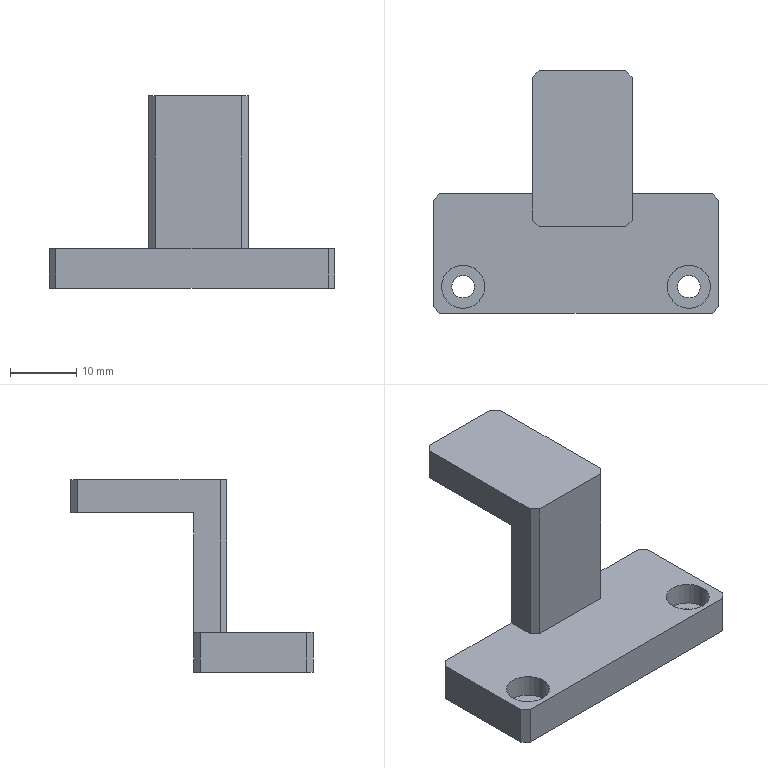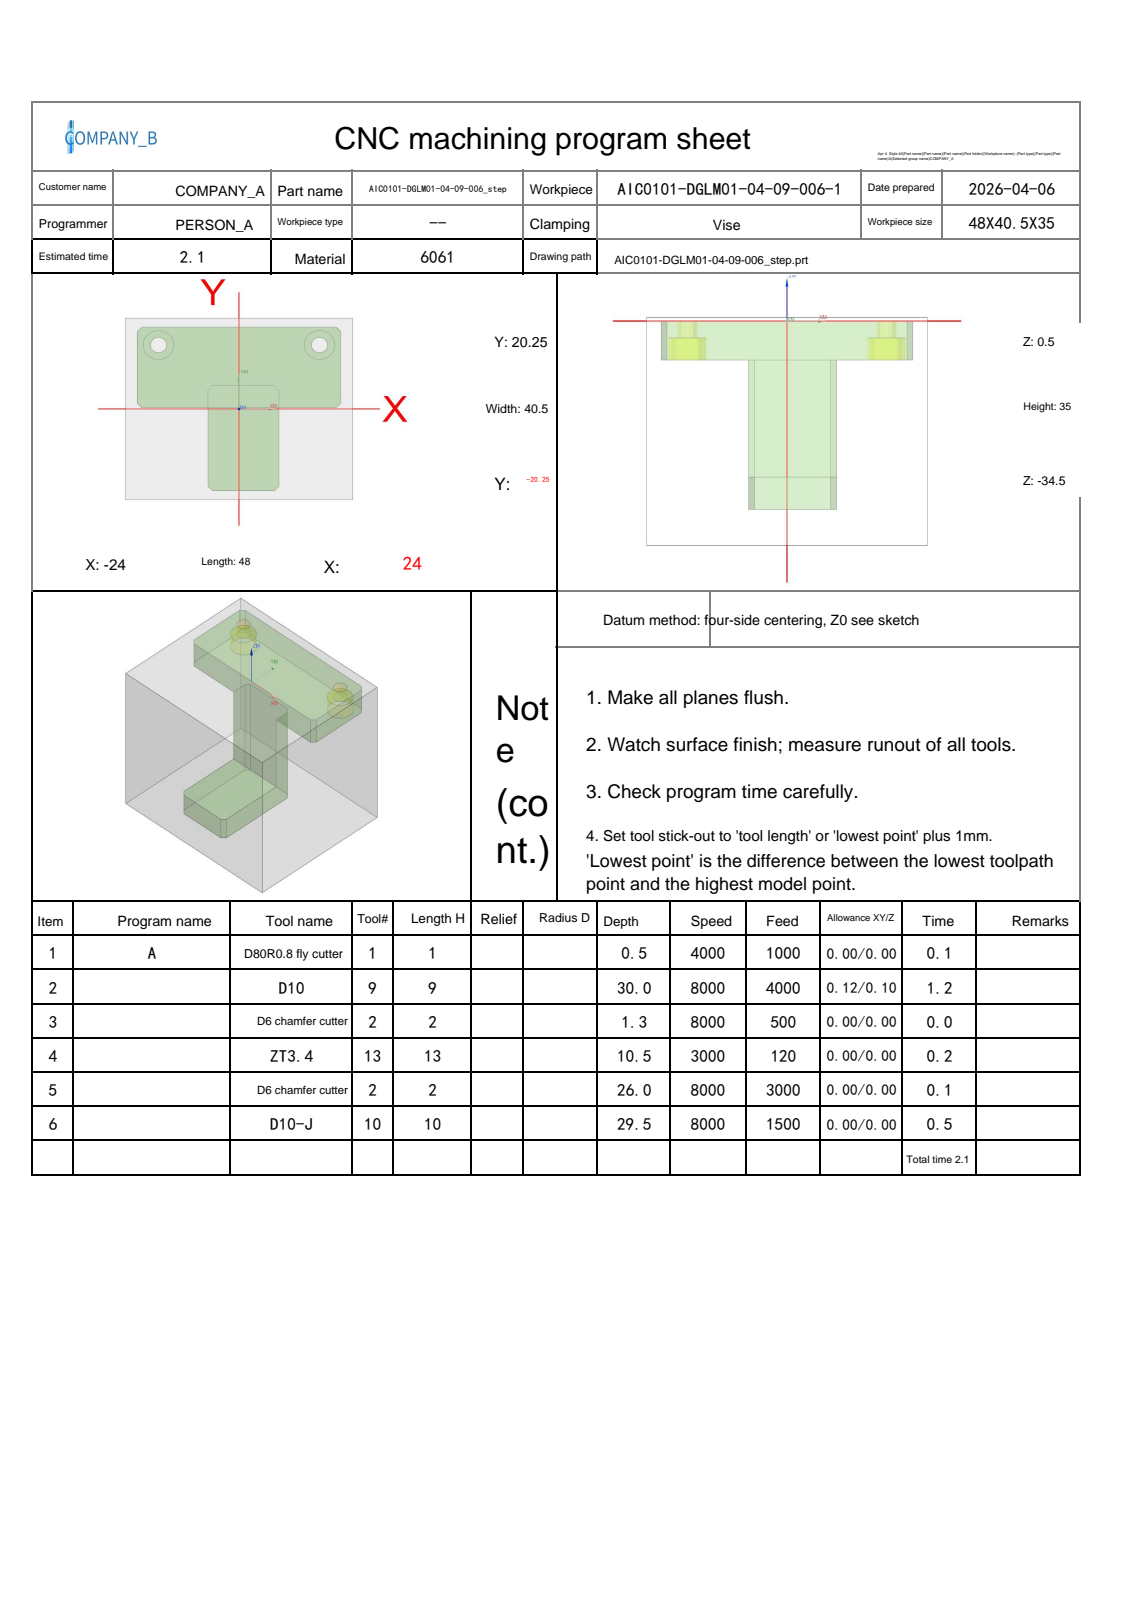NC program | NX | posted by the shop | part box 43 x 36.5 x 29 mm
Whole program, first 1428 of 1506 lines:
%
O0001
(Machine time: 3.30 MIN)
(===Total Tool:5===)
(T1=D80R0.8 fly cutter D=80.  R=0.8  D-  H01 Z=0.    )
(T9=D10     D=10.  R=0.   D-  H09 Z=-29.5 )
(T2=D6 chamfer cutter   D=6.   R=0.   D-  H02 Z=-25.5 )
(T13=ZT3.4  D=3.4  DR_a=118 D-  H13 Z=-10.  )
(T10=D10-J  D=10.  R=0.   D10 H10 Z=-29.  )
G80 G90 G17 G49 G40
G91 G28 Z0
M01
N1 T01 M06
(D80R0.8 fly cutter  D=80. R=0.8 H=01 ce=0.00 di=0.00)
G00 G90 G54 X66.5 Y0.0 M03 S4000
G43 H01 Z20.
M08
Z2.
G01 Z0.0 F1000.
X61.5
X-61.5
X-66.5
Z2.
G00 Z20.
G91 G28 Z0.0
M05
M09
G91 G28 Z0.0
M01
N2 T09 M06
(D10  D=10. R=0. H=09 ce=0.12 di=0.10)
G00 G90 G54 X34.981 Y10.037 M03 S8000
G43 H09 Z20.
M08
Z-12.75
G01 X34.882 Y10.019 Z-13.375 F4000.
X34.784 Y10. Z-13.622
X34.686 Y9.982 Z-13.804
X34.588 Y9.963 Z-13.95
X34.489 Y9.944 Z-14.073
X34.391 Y9.926 Z-14.178
X34.293 Y9.907 Z-14.27
X34.195 Y9.888 Z-14.35
X34.096 Y9.87 Z-14.42
X33.998 Y9.851 Z-14.482
X33.9 Y9.832 Z-14.536
X33.802 Y9.814 Z-14.583
X33.703 Y9.795 Z-14.624
X33.605 Y9.776 Z-14.658
X33.507 Y9.758 Z-14.686
X33.409 Y9.739 Z-14.71
X33.311 Y9.72 Z-14.727
X33.212 Y9.702 Z-14.74
X33.114 Y9.683 Z-14.747
X33.016 Y9.664 Z-14.75
X30.902 Y9.263
G03 X30.55 Y9.004 I.101 J-.505
X29.912 Y5.186 I12.295 J-4.018
X29.731 Y-4.985 I286.095 J-10.171
X29.75 Y-8.308 I286.276 J0.0
G02 X29.766 Y-11.961 I-421.132 J-3.653
X29.712 Y-18.707 I-421.148 J0.0
X25.772 Y-24.364 I-6.647 J.43
X19.798 Y-25.77 I-6.679 J14.988
X10.299 Y-26.019 I-9.499 J180.626
X7.563 Y-25.999 I0.0 J180.875
G01 X-22.16 Y-25.981
G02 X-28.142 Y-21.971 I.147 J6.684
X-29.511 Y-16.165 I14.924 J6.583
X-29.754 Y-8.022 I136.034 J8.142
X-29.745 Y-6.49 I136.278 J0.0
G01 X-29.724 Y18.53
G02 X-25.773 Y24.363 I6.664 J-.26
X-20.132 Y25.741 I6.523 J-14.467
X-11.878 Y26.006 I8.254 J-128.093
X-10.218 Y25.996 I0.0 J-128.359
G01 X22.14 Y25.982
G02 X28.113 Y22.022 I-.129 J-6.679
X29.498 Y16.301 I-14.573 J-6.557
X29.669 Y12.699 I-37.771 J-3.601
X29.34 Y7.712 I-37.942 J0.0
G03 X28.952 Y-2.655 I138.47 J-10.367
X28.958 Y-3.92 I138.858 J0.0
G02 X28.97 Y-7.922 I-674.054 J-4.002
X28.912 Y-16.768 I-674.066 J0.0
X24.873 Y-22.942 I-7.755 J.665
X18.704 Y-24.796 I-7.555 J13.945
X10.382 Y-25.192 I-8.321 J87.391
X9.357 Y-25.186 I0.0 J87.786
G01 X-20.237 Y-25.178
G02 X-26.758 Y-21.014 I.383 J7.787
X-28.561 Y-14.833 I14.332 J7.534
X-28.947 Y-6.277 I94.639 J8.555
X-28.938 Y-5.005 I95.025 J0.0
G01 X-28.925 Y16.547
G02 X-24.831 Y22.968 I7.771 J-.44
X-18.574 Y24.811 I7.579 J-14.18
X-10.101 Y25.196 I8.474 J-93.182
X-8.907 Y25.188 I0.0 J-93.567
G01 X20.297 Y25.175
G02 X26.672 Y21.155 I-.437 J-7.758
X28.549 Y14.914 I-13.851 J-7.568
X28.689 Y11.721 I-36.227 J-3.192
X28.562 Y8.682 I-36.367 J0.0
G03 X28.137 Y-6.178 I259.785 J-14.86
X28.151 Y-8.869 I260.21 J0.0
G02 X28.175 Y-10.971 I-92.316 J-2.103
X28.076 Y-15.246 I-92.34 J0.0
X23.277 Y-22.119 I-8.791 J1.026
X16.539 Y-24.001 I-8.189 J16.316
X7.13 Y-24.403 I-9.409 J110.137
X5.511 Y-24.391 I0.0 J110.538
G01 X-18.229 Y-24.381
G02 X-25.926 Y-19.425 I.261 J8.86
X-27.747 Y-12.832 I16.473 J8.098
X-28.154 Y-3.316 I111.108 J9.516
X-28.141 Y-1.644 I111.515 J0.0
X-28.167 Y5.086 I869.184 J6.729
X-28.113 Y14.816 I869.21 J0.0
X-25.197 Y20.784 I8.428 J-.421
X-23.358 Y22.498 I11.343 J-10.328
X-20.432 Y23.52 I4.026 J-6.829
X-11.841 Y24.338 I9.354 J-52.69
X-2.137 Y24.405 I9.704 J-701.618
X.798 Y24.399 I0.0 J-701.685
X7.757 Y24.423 I6.958 J-985.768
X18.538 Y24.364 I0.0 J-985.792
X24.467 Y21.543 I-.408 J-8.498
X26.793 Y17.745 I-5.173 J-5.781
X27.741 Y11.109 I-22.773 J-6.636
X27.714 Y9.995 I-23.72 J0.0
G03 X27.326 Y-12.789 I704.183 J-23.392
G02 X21.777 Y-21.338 I-9.682 J.21
X14.859 Y-23.185 I-8.544 J18.12
X5.047 Y-23.601 I-9.812 J115.406
X3.431 Y-23.59 I0.0 J115.823
G01 X-16.469 Y-23.577
G02 X-25.091 Y-18.024 I.135 J9.679
X-26.944 Y-11.02 I18.256 J8.579
X-27.349 Y-1.335 I115.699 J9.685
X-27.342 Y-.072 I116.103 J0.0
X-27.36 Y4.87 I668.627 J4.942
X-27.311 Y13.028 I668.646 J0.0
X-26.62 Y16.333 I11.421 J-.662
X-26.638 Y16.849 I7.56 J.516
X-26.379 Y18.811 I7.578 J0.0
X-25.164 Y20.819 I5.463 J-1.933
X-23.358 Y22.498 I10.236 J-9.204
X-20.511 Y23.37 I2.875 J-4.301
G03 X-19.772 Y23.369 I.739 J241.689
X-10.738 Y23.538 I0.0 J241.69
G02 X-.577 Y23.607 I10.161 J-745.963
X3.021 Y23.598 I0.0 J-746.032
X8.118 Y23.621 I5.096 J-573.355
X16.92 Y23.553 I0.0 J-573.378
G03 X19.639 Y23.349 I2.719 J17.97
X20.513 Y23.37 I0.0 J18.175
G02 X24.364 Y21.64 I-.152 J-5.492
G03 X20.513 Y23.37 I-3.985 J-3.721
G01 X-20.511
G03 X-23.358 Y22.498 I.028 J-5.173
X-25.558 Y20.372 I8.499 J-10.998
X-26.622 Y17.158 I4.32 J-3.214
G01 X-26.621 Y17.029
G03 X-26.701 Y6.045 I747.876 J-10.984
X-26.61 Y-5.658 I747.957 J0.0
X-25.746 Y-13.758 I41.101 J.29
X-22.709 Y-19.681 I12.069 J2.448
X-16.797 Y-22.493 I7.231 J7.583
X-9.947 Y-22.945 I6.85 J51.746
X-9.137 Y-22.938 I0.0 J52.198
X-2.61 Y-22.976 I6.527 J557.822
X10.381 Y-22.825 I0.0 J557.86
X18.295 Y-21.788 I-.489 J34.446
X24.073 Y-18.251 I-2.713 J10.917
X26.329 Y-12.509 I-9.036 J6.866
X26.716 Y-5.416 I-64.835 J7.093
G01 X26.715 Y-5.083
X27.045 Y10.295
Y10.317
G03 X26.618 Y15.139 I-27.439 J0.0
X26.643 Y16.073 I-17.638 J.934
X26.486 Y18.418 I-17.663 J0.0
G01 X26.154 Y19.384
G02 X26.618 Y17.401 I-4.878 J-2.187
G01 X26.603 Y.848
G03 X25.945 Y-5.754 I35.501 J-6.872
G02 X25.384 Y-12.442 I-43.977 J.321
X19.061 Y-20.17 I-10.225 J1.915
X11.678 Y-21.83 I-8.751 J21.676
X1.647 Y-22.163 I-10.031 J151.213
X-.154 Y-22.152 I0.0 J151.546
X-3.767 Y-22.179 I-3.613 J236.721
X-13.271 Y-21.989 I0.0 J236.749
X-18.863 Y-20.76 I.423 J15.263
X-24.081 Y-14.932 I4.836 J9.58
X-25.608 Y-7.599 I23.136 J8.641
X-25.871 Y-1.446 I146.918 J9.379
X-26.485 Y.069 I10.008 J4.937
G01 X-26.619 Y1.165
X-26.62 Y15.405
G03 X-27.12 Y15.905 I-.5 J0.0
X-27.542 Y15.673 I0.0 J-.5
G01 X-28.002 Y14.95
X-29.061 Y13.287 Z-14.65
X-29.287 Y12.932
X-29.321 Y12.869
X-29.345 Y12.802
X-29.36 Y12.732
X-29.365 Y12.66
X-29.279 Y.638
X-29.272 Y.56
X-29.253 Y.484
X-29.223 Y.412
X-29.182 Y.346
X-29.131 Y.287
X-29.072 Y.236
X-29.006 Y.196
X-27.21 Y-.618 Z-14.75
X-26.074 Y-1.138
G02 X-25.621 Y-2.196 I-1.372 J-1.215
X-24.923 Y-7.947 I-68.357 J-11.21
G03 X-23.154 Y-14.891 I21.428 J1.76
X-15.938 Y-20.622 I9.581 J4.655
X-8.569 Y-21.447 I7.369 J32.506
G01 X-8.479
G03 X-1.639 Y-21.533 I6.84 J271.025
X9.757 Y-21.294 I0.0 J271.111
X17.22 Y-19.995 I-.985 J27.764
X24.379 Y-12.214 I-3.311 J10.23
X25.247 Y-5.884 I-32.541 J7.689
G02 X25.599 Y-1.83 I87.405 J-5.549
G03 X26.445 Y.045 I-4.263 J3.05
G02 X25.577 Y-1.808 I-4.453 J.956
G03 X24.695 Y-5.125 I9.444 J-4.285
G02 X23.668 Y-11.157 I-50.122 J5.437
X16.62 Y-18.896 I-10.881 J2.83
X9.121 Y-20.418 I-8.85 J24.367
X-1.594 Y-20.726 I-10.715 J185.992
X-10.708 Y-20.503 I0.0 J186.3
X-16.929 Y-19.145 I.743 J18.327
X-22.668 Y-12.829 I4.837 J10.161
X-24.217 Y-6.144 I26.832 J9.74
G03 X-24.824 Y-2.726 I-28.743 J-3.344
G01 X-25.676 Y-1.712
X-25.879 Y-1.367
G03 X-24.791 Y-2.727 I6.377 J3.988
G02 X-23.761 Y-5.868 I-9.163 J-4.744
G03 X-22.177 Y-11.891 I36.569 J6.396
X-14.039 Y-19.064 I10.815 J4.067
X-6.431 Y-19.981 I7.782 J32.55
X-1.097 Y-20.073 I5.334 J154.977
X8.921 Y-19.749 I0.0 J155.069
X16.307 Y-18.107 I-1.317 J23.354
X22.761 Y-10.76 I-4.613 J10.561
X24.111 Y-4.749 I-52.898 J15.037
G02 X24.703 Y-2.788 I7.367 J-1.154
G03 X25.67 Y-1.685 I-8.228 J8.194
G02 X24.466 Y-3.057 I-15.953 J12.789
G03 X23.175 Y-6.327 I9.55 J-5.659
G02 X21.289 Y-11.754 I-26.032 J6.006
X14.245 Y-17.619 I-10.812 J5.824
X6.154 Y-19.037 I-9.176 J28.56
X-1.025 Y-19.25 I-7.179 J120.647
X-8.956 Y-18.99 I0.0 J120.86
X-15.523 Y-17.383 I1.049 J18.511
X-21.183 Y-11.153 I5.488 J10.672
X-22.997 Y-5.491 I42.708 J16.805
G03 X-23.663 Y-3.737 I-9.175 J-2.482
G02 X-24.88 Y-2.623 I8.816 J10.844
G03 X-23.71 Y-3.685 I5.639 J5.03
G02 X-22.542 Y-5.683 I-4.01 J-3.686
G03 X-20.489 Y-10.857 I60.394 J20.971
X-12.281 Y-17.529 I11.203 J5.397
X-4.361 Y-18.515 I8.12 J32.916
X-.662 Y-18.59 I3.699 J91.438
X8.582 Y-18.122 I0.0 J91.512
X15.753 Y-16.002 I-1.841 J19.411
X21.249 Y-9.542 I-6.435 J11.043
X23.011 Y-4.811 I-543.409 J205.171
G02 X24.119 Y-3.371 I2.395 J-.696
G01 X24.629 Y-2.862
G02 X23.181 Y-4.162 I-15.904 J16.255
G03 X21.546 Y-7.02 I9.61 J-7.395
G02 X18.651 Y-12.032 I-19.74 J8.059
X11.224 Y-16.55 I-10.823 J9.427
X2.115 Y-17.681 I-9.449 J38.866
X-1.04 Y-17.757 I-3.155 J65.214
X-8.825 Y-17.291 I0.0 J65.29
X-15.589 Y-14.79 I1.755 J15.144
X-20.121 Y-9.052 I8.884 J11.676
G03 X-22.177 Y-4.803 I-51.324 J-22.211
X-23.055 Y-4.187 I-1.147 J-.701
G01 X-23.69 Y-3.701
G03 X-22.392 Y-4.47 I2.359 J2.502
G02 X-20.645 Y-6.845 I-5.459 J-5.845
G03 X-17.634 Y-11.627 I26.19 J13.148
X-9.829 Y-16.219 I10.638 J9.154
X-1.534 Y-17.059 I8.295 J40.511
X-.606 Y-17.049 I0.0 J41.351
X.349 Y-17.058 I.955 J49.283
X9.264 Y-16.245 I0.0 J49.293
X16.701 Y-12.673 I-2.722 J15.195
X20.416 Y-7.588 I-13.265 J13.592
G02 X22.301 Y-4.564 I14.803 J-7.127
G01 X23.313 Y-4.028
G03 X21.785 Y-4.903 I2.938 J-6.904
X19.432 Y-7.93 I13.075 J-12.592
G02 X13.826 Y-13.38 I-14.256 J9.056
X5.832 Y-15.807 I-10.133 J18.995
X-.511 Y-16.209 I-6.343 J49.791
X-7.726 Y-15.688 I0.0 J50.193
X-15.379 Y-12.245 I2.112 J14.92
X-18.913 Y-7.935 I14.165 J15.216
G03 X-21.187 Y-4.869 I-15.99 J-9.488
X-21.822 Y-4.696 I-.653 J-1.143
G01 X-22.488 Y-4.421
G03 X-21.281 Y-4.778 I1.458 J2.711
G02 X-19.229 Y-6.691 I-3.492 J-5.805
G03 X-15.584 Y-10.953 I29.604 J21.622
X-7.233 Y-14.927 I10.884 J12.11
X-.277 Y-15.501 I6.956 J41.888
X8.198 Y-14.647 I0.0 J42.461
X18.098 Y-8.38 I-3.457 J16.415
G02 X20.908 Y-5.084 I24.963 J-18.441
X21.385 Y-4.793 I.877 J-.898
G01 X22.386 Y-4.51
G03 X20.686 Y-5.055 I1.577 J-7.84
X18.386 Y-7.065 I6.867 J-10.178
G02 X13.427 Y-11.38 I-18.981 J16.806
X4.593 Y-14.274 I-11.013 J18.685
X-.345 Y-14.61 I-4.938 J36.139
X-7.427 Y-13.916 I0.0 J36.475
X-16.494 Y-8.492 I3.671 J16.426
G03 X-19.613 Y-5.262 I-25.893 J-21.883
X-20.494 Y-4.87 I-.881 J-.793
G01 X-20.502
X-21.374 Y-4.755
G02 X-19.94 Y-4.94 I-.772 J-11.62
X-17.47 Y-6.742 I-3.733 J-7.712
G03 X-13.001 Y-10.597 I24.276 J23.625
X-4.076 Y-13.645 I10.613 J16.481
X-.2 Y-13.877 I3.876 J32.271
X8.529 Y-12.683 I0.0 J32.503
X16.472 Y-7.912 I-5.993 J18.972
G02 X19.745 Y-5.122 I17.833 J-17.61
X20.562 Y-4.851 I.817 J-1.097
G01 X20.734 Y-4.862
X21.298 Y-4.805
X19.943 Y-4.907
G03 X17.222 Y-6.459 I2.675 J-7.85
G02 X12.097 Y-10.07 I-25.484 J30.736
X1.676 Y-12.867 I-11.401 J21.66
X-.437 Y-12.952 I-2.112 J26.145
X-8.356 Y-11.728 I0.0 J26.23
X-15.136 Y-7.635 I7.191 J19.571
G03 X-18.527 Y-5.038 I-15.74 J-17.045
G01 X-18.953 Y-4.87
X-20.233
G02 X-19.641 Y-4.848 I.592 J-7.874
X-18.578 Y-4.919 I0.0 J-7.897
X-15.546 Y-6.648 I-3.491 J-9.643
G03 X-9.836 Y-10.253 I19.364 J24.346
X-.376 Y-12.185 I9.46 J22.204
X1.108 Y-12.139 I0.0 J24.136
X14.735 Y-7.433 I-.549 J23.668
G02 X18.515 Y-5.001 I15.652 J-20.174
G01 X18.891 Y-4.87
X20.251
G03 X19.588 Y-4.846 I-.662 J-9.127
X18.125 Y-4.964 I0.0 J-9.151
X14.854 Y-6.562 I4.535 J-13.429
G02 X7.432 Y-10.116 I-17.225 J26.449
X.023 Y-11.226 I-7.409 J24.169
X-7.39 Y-10.115 I0.0 J25.279
X-13.781 Y-6.81 I8.814 J24.874
G03 X-17.111 Y-4.88 I-11.152 J-15.409
G01 X-18.93 Y-4.87
X-18.67 Y-4.869
G02 X-16.806 Y-4.902 I0.0 J-53.437
X-13.466 Y-6.398 I-3.432 J-12.135
G03 X-6.501 Y-9.558 I15.915 J25.829
X0.0 Y-10.41 I6.5 J24.356
X12.598 Y-7.036 I0.0 J25.208
G02 X16.888 Y-4.887 I17.173 J-28.917
G01 X18.661 Y-4.87
G03 X17.842 Y-4.849 I-.82 J-16.085
X16.123 Y-4.941 I0.0 J-16.106
X12.971 Y-6.105 I4.107 J-15.979
G02 X5.338 Y-8.874 I-16.37 J33.215
X.127 Y-9.45 I-5.212 J23.303
X-11.124 Y-6.633 I0.0 J23.878
G03 X-14.912 Y-4.87 I-14.665 J-26.559
G01 X-17.152
G02 X-16.202 Y-4.853 I.95 J-27.136
X-14.356 Y-4.916 I0.0 J-27.153
X-10.304 Y-6.377 I-5.711 J-22.181
G03 X.185 Y-8.645 I10.49 J23.122
X2.008 Y-8.58 I0.0 J25.39
X11.019 Y-6.196 I-2.915 J29.235
G02 X14.493 Y-4.87 I15.786 J-36.157
G01 X16.733
G03 X15.575 Y-4.846 I-1.158 J-27.595
X13.37 Y-4.934 I0.0 J-27.619
X8.71 Y-6.266 I9.067 J-40.532
G02 X.181 Y-7.666 I-8.529 J25.275
X-2.81 Y-7.498 I0.0 J26.675
X-10.391 Y-5.405 I5.127 J33.339
G01 X-11.965 Y-4.87
X-14.765
G02 X-13.475 Y-4.846 I1.29 J-34.378
X-11.042 Y-4.932 I0.0 J-34.403
X-6.143 Y-6.139 I-17.68 J-82.285
G03 X.145 Y-6.894 I6.287 J25.823
X7.614 Y-5.822 I0.0 J26.577
G01 X11.069 Y-4.87
X13.949
G03 X12.284 Y-4.845 I-1.665 J-56.462
X9.355 Y-4.921 I0.0 J-56.486
G02 X3.102 Y-5.848 I-45.905 J288.102
X.572 Y-5.951 I-2.53 J31.225
X-7.546 Y-4.88 I0.0 J31.327
G01 X-11.685 Y-4.87
G02 X-9.508 Y-4.847 I2.177 J-101.533
X-5.36 Y-4.931 I0.0 J-101.557
G03 X-.286 Y-5.23 I5.075 J42.985
X3.149 Y-5.093 I0.0 J43.284
G01 X5.067 Y-4.87
X10.107
X-6.453
G03 X-6.955 Y-5.317 I.001 J-.506
G01 X-7.189 Y-7.332
X-7.2 Y-7.431 Z-14.747
X-7.212 Y-7.531 Z-14.74
X-7.223 Y-7.63 Z-14.727
X-7.235 Y-7.729 Z-14.71
X-7.246 Y-7.829 Z-14.686
X-7.258 Y-7.928 Z-14.658
X-7.269 Y-8.027 Z-14.624
X-7.281 Y-8.127 Z-14.583
X-7.292 Y-8.226 Z-14.536
X-7.304 Y-8.325 Z-14.482
X-7.315 Y-8.425 Z-14.42
X-7.327 Y-8.524 Z-14.35
X-7.338 Y-8.623 Z-14.27
X-7.35 Y-8.723 Z-14.178
X-7.361 Y-8.822 Z-14.073
X-7.373 Y-8.921 Z-13.95
X-7.384 Y-9.021 Z-13.804
X-7.396 Y-9.12 Z-13.622
X-7.407 Y-9.219 Z-13.375
X-7.419 Y-9.319 Z-12.75
G00 Z20.
X34.931 Y10.059
Z-27.5
G01 X34.832 Y10.041 Z-28.125
X34.734 Y10.022 Z-28.372
X34.636 Y10.003 Z-28.554
X34.538 Y9.985 Z-28.7
X34.439 Y9.966 Z-28.823
X34.341 Y9.947 Z-28.928
X34.243 Y9.929 Z-29.02
X34.145 Y9.91 Z-29.1
X34.046 Y9.891 Z-29.17
X33.948 Y9.873 Z-29.232
X33.85 Y9.854 Z-29.286
X33.752 Y9.835 Z-29.333
X33.653 Y9.817 Z-29.374
X33.555 Y9.798 Z-29.408
X33.457 Y9.779 Z-29.436
X33.359 Y9.76 Z-29.46
X33.26 Y9.742 Z-29.477
X33.162 Y9.723 Z-29.49
X33.064 Y9.704 Z-29.497
X32.966 Y9.686 Z-29.5
X30.851 Y9.284
G03 X30.5 Y9.025 I.101 J-.505
X29.862 Y5.215 I12.241 J-4.008
X29.681 Y-4.953 I285.25 J-10.168
X29.7 Y-8.278 I285.431 J0.0
G02 X29.724 Y-12.282 I-340.099 J-4.003
X29.664 Y-18.677 I-340.123 J0.0
X25.83 Y-24.268 I-6.588 J.408
X19.878 Y-25.71 I-6.684 J14.579
X11.771 Y-25.954 I-8.107 J134.991
X10.284 Y-25.945 I0.0 J135.234
G01 X-22.13 Y-25.932
G02 X-28.067 Y-21.992 I.136 J6.646
X-29.449 Y-16.271 I14.6 J6.554
X-29.713 Y-7.575 I143.083 J8.695
X-29.697 Y-5.476 I143.347 J0.0
G01 X-29.676 Y18.5
G02 X-25.87 Y24.245 I6.593 J-.234
X-20.239 Y25.677 I6.537 J-13.917
X-11.501 Y25.964 I8.738 J-133.
X-9.366 Y25.947 I0.0 J-133.287
G01 X22.25 Y25.926
G02 X28.025 Y22.061 I-.244 J-6.611
X29.461 Y16.111 I-14.611 J-6.676
X29.617 Y12.689 I-37.477 J-3.421
X29.29 Y7.742 I-37.633 J0.0
G03 X28.903 Y-2.627 I138.383 J-10.369
X28.908 Y-3.89 I138.771 J0.0
G02 X28.92 Y-7.889 I-680.254 J-3.999
X28.862 Y-16.738 I-680.266 J0.0
X24.74 Y-22.947 I-7.759 J.678
X18.64 Y-24.75 I-7.505 J14.175
X10.084 Y-25.147 I-8.556 J91.951
X8.813 Y-25.138 I0.0 J92.348
G01 X-20.207 Y-25.129
G02 X-26.68 Y-21.024 I.381 J7.756
X-28.524 Y-14.688 I14.338 J7.609
X-28.906 Y-5.743 I104.585 J8.945
X-28.892 Y-4.059 I104.966 J0.0
G01 X-28.877 Y16.497
G02 X-24.805 Y22.909 I7.751 J-.424
X-18.157 Y24.812 I7.734 J-14.453
X-9.557 Y25.149 I8.6 J-109.463
X-8.246 Y25.141 I0.0 J-109.801
G01 X20.167 Y25.131
G02 X26.629 Y21.102 I-.342 J-7.744
X28.525 Y14.62 I-14.066 J-7.632
X28.633 Y11.801 I-36.58 J-2.818
X28.528 Y9.026 I-36.688 J0.0
G03 X28.088 Y-6.194 I262.708 J-15.219
X28.101 Y-8.839 I263.149 J0.0
G02 X28.125 Y-10.946 I-91.38 J-2.108
X28.025 Y-15.216 I-91.404 J0.0
X23.079 Y-22.154 I-8.815 J1.053
X16.395 Y-23.964 I-8.13 J16.776
X7.192 Y-24.35 I-9.202 J109.512
X6.566 Y-24.348 I0.0 J109.898
G01 X-18.167 Y-24.333
G02 X-25.851 Y-19.431 I.236 J8.844
X-27.7 Y-12.763 I16.413 J8.143
X-28.096 Y-3.683 I103.921 J9.08
X-28.088 Y-2.375 I104.317 J0.0
X-28.119 Y5.056 I895.136 J7.431
X-28.066 Y14.725 I895.166 J0.0
X-25.557 Y20.373 I8.481 J-.386
X-23.358 Y22.498 I11.504 J-9.706
X-20.429 Y23.506 I3.876 J-6.501
X-11.434 Y24.293 I9.423 J-55.937
X-4.929 Y24.356 I6.504 J-332.928
X-2.734 Y24.349 I0.0 J-332.991
G01 X18.526 Y24.326
G02 X24.121 Y21.87 I-.606 J-8.984
X26.154 Y19.384 I-5.299 J-6.408
X27.674 Y11.695 I-18.689 J-7.689
X27.669 Y11.263 I-20.208 J0.0
X27.367 Y-.834 I-920.548 J16.946
G01 X27.276 Y-12.759
G02 X21.723 Y-21.294 I-9.672 J.219
X14.557 Y-23.163 I-8.646 J18.473
X5.241 Y-23.545 I-9.316 J113.466
X4.008 Y-23.538 I0.0 J113.848
G01 X-16.532 Y-23.523
G02 X-25.055 Y-17.953 I.24 J9.673
X-26.898 Y-10.95 I18.347 J8.573
X-27.297 Y-1.384 I114.431 J9.566
X-27.291 Y-.242 I114.83 J0.0
X-27.309 Y4.832 I731.067 J5.074
X-27.264 Y12.938 I731.084 J0.0
X-26.62 Y16.164 I11.596 J-.637
X-26.643 Y16.769 I8.024 J.604
X-26.379 Y18.811 I8.047 J0.0
X-25.57 Y20.354 I5.567 J-1.935
G03 X-26.626 Y17.143 I4.35 J-3.211
G01 X-26.623 Y16.944
X-26.601 Y-3.795
X-26.602 Y-4.088
G03 X-25.91 Y-12.718 I54.192 J0.0
X-23.299 Y-18.922 I13.722 J2.125
X-17.291 Y-22.344 I7.6 J6.359
X-10.54 Y-22.885 I6.751 J41.837
X-9.88 Y-22.88 I0.0 J42.378
G01 X-7.529 Y-22.925
X-6.875 Y-23.196
X-5.552 Y-23.37
X7.448
G02 X14.94 Y-22.438 I33.581 J-239.351
G03 X21.393 Y-20.432 I-1.939 J17.622
X26.105 Y-13.495 I-4.987 J8.455
X26.64 Y-6.798 I-41.639 J6.696
X26.639 Y-6.484 I-42.174 J0.0
G02 X26.998 Y9.674 I998.354 J-14.148
G03 X27.002 Y10.16 I-29.997 J.486
X26.618 Y14.947 I-30.001 J0.0
G01 Y17.401
G03 X26.154 Y19.384 I-5.342 J-.204
G02 X26.618 Y17.401 I-4.879 J-2.187
G01 X26.62 Y1.373
G02 X26.333 Y-.454 I-6.381 J.066
G03 X25.843 Y-7.087 I54.645 J-7.374
G02 X25.128 Y-13.273 I-28.89 J.203
X19.125 Y-20.083 I-10.011 J2.774
X12.41 Y-21.825 I-9.565 J23.057
G01 X10.802 Y-22.095
X10.01 Y-22.684
X8.775 Y-23.196
X10.01 Y-22.684
G02 X12.538 Y-21.415 I3.644 J-4.106
G03 X18.031 Y-19.686 I-8.646 J37.065
X24.335 Y-12.169 I-4.259 J9.974
X25.174 Y-6.238 I-31.415 J7.472
G02 X25.574 Y-1.851 I63.38 J-3.559
G03 X26.369 Y-.265 I-4.401 J3.2
G02 X25.443 Y-2.029 I-5.926 J1.987
G03 X24.58 Y-5.621 I12.334 J-4.864
G02 X23.494 Y-11.563 I-38.391 J3.947
X17.231 Y-18.7 I-10.998 J3.335
X12.35 Y-20.629 I-26.307 J59.426
G03 X11.069 Y-21.871 I7.459 J-8.971
G01 X10.752 Y-22.115
G03 X12.244 Y-20.655 I-5.978 J7.602
G02 X14.502 Y-19.33 I6.917 J-9.2
G03 X19.455 Y-16.19 I-7.418 J17.181
X23.026 Y-9.753 I-9.436 J9.442
X24.207 Y-4.184 I-214.008 J48.328
G02 X24.665 Y-2.826 I6.089 J-1.294
G03 X25.62 Y-1.747 I-7.914 J7.973
G02 X24.44 Y-3.077 I-13.916 J11.166
G03 X23.167 Y-6.232 I8.946 J-5.443
G02 X21.402 Y-11.515 I-30.124 J7.13
X16.001 Y-17.324 I-12.636 J6.334
G03 X13.22 Y-19.11 I73.42 J-117.386
X12.884 Y-19.81 I3.389 J-2.054
G01 X12.153 Y-20.762
G03 X13.184 Y-19.11 I-3.624 J3.408
G02 X14.916 Y-17.494 I7.434 J-6.229
G03 X19.299 Y-13.252 I-12.058 J16.844
X22.081 Y-7.333 I-17.941 J12.047
G02 X23.395 Y-3.984 I20.878 J-6.261
G03 X24.572 Y-2.919 I-16.295 J19.187
G02 X23.172 Y-4.168 I-16.403 J16.978
G03 X21.489 Y-7.151 I9.216 J-7.164
G02 X18.221 Y-12.954 I-22.595 J8.905
X14.284 Y-16.918 I-31.986 J27.826
G03 X13.486 Y-17.892 I1.808 J-2.298
G02 X13.12 Y-19.24 I-2.904 J.063
G03 X13.516 Y-17.735 I-3.266 J1.663
G02 X15.363 Y-15.235 I8.922 J-4.661
G03 X20.691 Y-7.231 I-21.99 J20.412
G02 X22.351 Y-4.533 I10.295 J-4.473
G01 X23.312 Y-4.028
G03 X21.621 Y-5.082 I2.227 J-5.458
X19.777 Y-7.652 I11.938 J-10.517
G02 X14.73 Y-14.699 I-43.899 J26.109
G03 X13.588 Y-16.417 I7.779 J-6.407
G02 X13.486 Y-17.886 I-11.598 J.064
G03 X13.58 Y-16.605 I-8.708 J1.281
X13.576 Y-16.355 I-8.802 J0.0
G02 X14.846 Y-13.857 I7.567 J-2.273
G03 X19.748 Y-6.574 I-265.94 J184.274
G02 X21.388 Y-4.792 I5.531 J-3.447
G01 X22.388 Y-4.509
G03 X20.776 Y-5.069 I1.142 J-5.896
X18.178 Y-7.809 I6.873 J-9.117
X14.01 Y-13.848 I58.505 J-44.832
X13.57 Y-14.816 I5.803 J-3.222
G01 Y-16.496
G02 X13.56 Y-15.848 I21.162 J.648
X13.607 Y-14.437 I21.172 J0.0
X15.157 Y-11.168 I10.906 J-3.168
X19.114 Y-5.871 I26.762 J-15.869
X20.448 Y-4.884 I3.797 J-3.732
G01 X21.384 Y-4.793
G03 X20.062 Y-4.955 I.359 J-8.412
X17.401 Y-7.011 I3.063 J-6.713
X13.589 Y-12.737 I15.83 J-14.669
G01 X13.57 Y-14.759
X13.598 Y-12.461
G02 X15.434 Y-8.676 I10.414 J-2.713
X18.795 Y-5.189 I10.475 J-6.734
X19.491 Y-4.87 I1.842 J-3.099
G01 X20.406
G03 X19.949 Y-4.846 I-.457 J-4.273
X18.651 Y-5.046 I0.0 J-4.298
X15.332 Y-7.849 I3.959 J-8.054
X13.57 Y-10.856 I7.867 J-6.631
G01 Y-12.696
X13.596 Y-10.498
G02 X16.104 Y-6.337 I8.404 J-2.228
X18.284 Y-4.87 I4.174 J-3.849
G01 X19.404
G03 X18.864 Y-4.846 I-.539 J-5.985
X17.586 Y-4.983 I0.0 J-6.009
X14.093 Y-8.051 I2.782 J-6.691
X13.57 Y-9.117 I4.213 J-2.727
G01 Y-10.797
G02 X13.552 Y-10.07 I14.887 J.727
X13.611 Y-8.745 I14.905 J0.0
X17.001 Y-4.885 I5.893 J-1.756
G01 X18.13 Y-4.87
G03 X17.628 Y-4.846 I-.502 J-5.343
X16.378 Y-4.994 I0.0 J-5.367
X13.578 Y-7.721 I1.921 J-4.774
G01 X13.57 Y-9.044
G02 X13.552 Y-8.489 I8.349 J.555
X13.623 Y-7.395 I8.367 J0.0
X16.032 Y-4.87 I3.798 J-1.212
G01 X16.992
G03 X16.533 Y-4.85 I-.459 J-5.197
X15.509 Y-4.951 I0.0 J-5.218
X13.587 Y-6.693 I1.175 J-3.227
G01 X13.57 Y-7.748
G02 X13.549 Y-7.313 I4.451 J.434
X13.639 Y-6.418 I4.472 J0.0
X15.218 Y-4.87 I2.414 J-.883
G01 X15.938
G03 X15.58 Y-4.846 I-.358 J-2.66
X14.515 Y-5.066 I0.0 J-2.684
X13.57 Y-6.141 I.711 J-1.577
G01 Y-6.781
G02 X13.546 Y-6.452 I2.246 J.329
X13.644 Y-5.791 I2.27 J0.0
X14.671 Y-4.87 I1.491 J-.63
G01 X15.151
G03 X14.884 Y-4.846 I-.266 J-1.458
X13.6 Y-5.588 I0.0 J-1.482
G01 X13.57 Y-6.123
G02 X13.548 Y-5.907 I1.066 J.216
X14.308 Y-4.87 I1.087 J0.0
G01 X14.628
G03 X14.42 Y-4.845 I-.209 J-.862
X13.57 Y-5.477 I0.0 J-.887
G01 Y-5.797
G03 X14.12 Y-6.346 I.55 J0.0
X14.649 Y-5.949 I0.0 J.55
G01 X14.73 Y-5.68
X14.778 Y-5.404
G03 X14.228 Y-4.87 I-.551 J-.016
G01 X14.184 Y-4.868
G03 X13.581 Y-5.421 I0.0 J-.605
G01 X13.572 Y-5.518
G03 X13.756 Y-5.907 I.505 J0.0
G01 X14.501 Y-6.514
X16.029 Y-7.759 Z-29.4
X16.534 Y-8.17
X16.588 Y-8.221
X16.633 Y-8.279
X16.67 Y-8.343
X16.696 Y-8.412
X16.713 Y-8.484
X16.718 Y-8.558
Y-19.394
X16.712 Y-19.611
X16.692 Y-19.827
X16.659 Y-20.041
X16.614 Y-20.253
X16.556 Y-20.462
X16.485 Y-20.667
X16.402 Y-20.867
X16.307 Y-21.062
X16.2 Y-21.251
X16.083 Y-21.433
X15.954 Y-21.608
X15.815 Y-21.775
X15.667 Y-21.932
X14.104 Y-23.495
X13.852 Y-23.738
X13.591 Y-23.971
X13.321 Y-24.194
X13.043 Y-24.407
X12.757 Y-24.609
X12.464 Y-24.801
X12.164 Y-24.981
X11.806 Y-25.179
X11.441 Y-25.364
X11.07 Y-25.537
X10.693 Y-25.696
X10.311 Y-25.843
X9.924 Y-25.977
X9.59 Y-26.078
X9.251 Y-26.166
X8.909 Y-26.24
X8.565 Y-26.3
X8.218 Y-26.345
X7.87 Y-26.377
X7.521 Y-26.394
X-5.31 Y-26.767
X-5.394 Y-26.762
X-5.476 Y-26.744
X-5.554 Y-26.712
X-5.625 Y-26.667
X-5.687 Y-26.611
X-5.74 Y-26.546
X-5.781 Y-26.473
X-6.079 Y-25.81
X-6.889 Y-24.013 Z-29.5
X-7.3 Y-23.115
G03 X-8.438 Y-22.616 I-1.395 J-1.633
X-13.787 Y-21.966 I-8.408 J-46.847
G02 X-19.238 Y-20.513 I.903 J14.344
X-24.184 Y-14.508 I5.502 J9.57
X-25.622 Y-6.668 I25.882 J8.799
X-25.805 Y-1.553 I402.995 J17.015
X-26.485 Y.069 I8.391 J4.472
G01 X-26.619 Y1.165
G03 X-25.774 Y-1.561 I5.45 J.197
G02 X-25.159 Y-5.148 I-15.677 J-4.53
G03 X-24.14 Y-12.013 I43.755 J2.991
X-20.721 Y-18.087 I11.884 J2.691
X-14.919 Y-20.871 I8.116 J9.477
X-9.593 Y-21.798 I48.141 J260.678
G01 X-9.057 Y-21.957
G03 X-7.888 Y-22.776 I3.473 J3.714
G02 X-9.057 Y-21.957 I2.304 J4.533
G03 X-11.715 Y-20.885 I-4.145 J-6.449
G02 X-16.716 Y-19.313 I6.294 J28.762
X-22.673 Y-12.689 I4.986 J10.475
X-24.119 Y-6.469 I26.699 J9.487
G03 X-24.808 Y-2.719 I-22.259 J-2.151
G02 X-25.838 Y-1.437 I5.665 J5.605
G03 X-24.751 Y-2.767 I6.913 J4.538
G02 X-23.751 Y-5.714 I-8.549 J-4.545
G03 X-22.201 Y-11.707 I40.794 J7.354
X-14.978 Y-18.986 I11.466 J4.156
G02 X-10.449 Y-20.665 I-83.115 J-231.128
G01 X-10.171 Y-20.869
X-9.172 Y-21.869
G03 X-10.726 Y-20.336 I-16.502 J-15.174
X-14.226 Y-18.487 I-14.545 J-23.302
G02 X-21.473 Y-10.416 I5.819 J12.514
X-23.127 Y-4.971 I106.285 J35.256
G03 X-23.671 Y-3.715 I-4.094 J-1.028
G02 X-24.825 Y-2.681 I6.008 J7.861
G03 X-23.671 Y-3.715 I5.42 J4.884
G02 X-22.513 Y-5.681 I-3.843 J-3.589
G03 X-20.48 Y-10.902 I73.586 J25.641
X-14.205 Y-17.534 I13.496 J6.486
G02 X-11.219 Y-19.366 I-21.502 J-38.393
G03 X-10.205 Y-20.825 I7.612 J4.208
G01 X-10.984 Y-19.81
G03 X-12.158 Y-18.311 I-3.129 J-1.241
G02 X-16.104 Y-15.093 I40.494 J53.692
X-20.435 Y-8.497 I13.719 J13.726
G03 X-22.304 Y-4.595 I-24.836 J-9.498
X-23.056 Y-4.187 I-1.097 J-1.124
G01 X-23.627 Y-3.749
G03 X-22.371 Y-4.48 I2.32 J2.542
G02 X-20.628 Y-6.919 I-5.392 J-5.696
G03 X-17.511 Y-12.25 I33.641 J16.093
X-12.909 Y-16.827 I23.052 J18.578
G02 X-11.569 Y-18.194 I-5.507 J-6.737
G03 X-11.128 Y-19.462 I4.38 J.813
G02 X-11.558 Y-18.147 I3.431 J1.849
G03 X-13.126 Y-15.941 I-6.733 J-3.126
G02 X-19.378 Y-7.462 I25.839 J25.597
G03 X-21.303 Y-4.814 I-9.659 J-4.999
X-21.823 Y-4.696 I-.877 J-2.672
G01 X-22.488 Y-4.421
G03 X-21.326 Y-4.772 I1.433 J2.645
G02 X-19.321 Y-6.762 I-3.266 J-5.293
G03 X-15.482 Y-12.192 I83.132 J54.712
G02 X-12.119 Y-16.254 I-76.349 J-66.635
X-11.67 Y-17.248 I-1.22 J-1.149
G01 X-11.534 Y-18.279
G03 X-11.756 Y-16.565 I-19.935 J-1.708
X-13.515 Y-13.571 I-10.879 J-4.377
G02 X-18.364 Y-6.814 I711.301 J515.543
G03 X-20.316 Y-4.898 I-5.781 J-3.939
G01 X-21.453 Y-4.745
G02 X-20.083 Y-4.951 I-.316 J-6.762
X-17.582 Y-7.122 I-3.651 J-6.732
X-12.323 Y-14.297 I-66.948 J-54.578
X-11.67 Y-15.679 I-6.168 J-3.761
G01 Y-17.039
G03 X-11.647 Y-16.378 I-9.435 J.661
X-11.761 Y-14.91 I-9.458 J0.0
X-13.592 Y-11.315 I-12.851 J-4.277
X-17.741 Y-5.977 I-27.544 J-17.129
X-19.277 Y-4.883 I-3.954 J-3.926
G01 X-20.4 Y-4.87
G02 X-19.901 Y-4.846 I.499 J-5.166
X-18.999 Y-4.925 I0.0 J-5.19
X-16.313 Y-6.884 I-2.692 J-6.512
X-11.807 Y-13.44 I-18.039 J-17.226
G01 X-11.67 Y-13.849
Y-15.449
G03 X-11.649 Y-14.64 I-15.527 J.809
X-11.718 Y-13.172 I-15.548 J0.0
X-13.747 Y-9.02 I-11.723 J-3.155
X-17.339 Y-5.225 I-11.919 J-7.686
X-18.07 Y-4.87 I-1.594 J-2.349
G01 X-19.35
G02 X-18.801 Y-4.855 I.549 J-10.238
X-17.758 Y-4.908 I0.0 J-10.253
X-14.866 Y-6.903 I-2.33 J-6.474
X-11.67 Y-11.883 I-9.951 J-9.9
G01 Y-13.563
G03 X-11.652 Y-12.758 I-17.563 J.805
X-11.722 Y-11.181 I-17.581 J0.0
X-14.404 Y-6.561 I-9.866 J-2.637
X-16.64 Y-4.887 I-5.421 J-4.911
G01 X-18.015 Y-4.87
G02 X-17.445 Y-4.851 I.57 J-8.817
X-16.378 Y-4.916 I0.0 J-8.836
X-13.33 Y-7.183 I-2.343 J-6.334
X-11.67 Y-10.029 I-6.811 J-5.88
G01 Y-11.629
G03 X-11.648 Y-10.844 I-14.159 J.785
X-11.721 Y-9.409 I-14.18 J0.0
X-15.347 Y-4.89 I-6.9 J-1.824
G01 X-16.732 Y-4.87
G02 X-16.174 Y-4.851 I.558 J-8.163
X-15.082 Y-4.924 I0.0 J-8.182
X-11.67 Y-8.493 I-2.111 J-5.433
G01 Y-9.853
G03 X-11.647 Y-9.193 I-9.321 J.661
X-11.742 Y-7.863 I-9.344 J0.0
X-14.254 Y-4.885 I-4.681 J-1.401
G01 X-15.384 Y-4.87
G02 X-14.926 Y-4.852 I.458 J-5.892
X-13.983 Y-4.928 I0.0 J-5.91
X-11.67 Y-7.306 I-1.36 J-3.637
G01 Y-8.266
G03 X-11.646 Y-7.795 I-4.599 J.471
X-11.802 Y-6.605 I-4.623 J0.0
X-13.388 Y-4.885 I-2.965 J-1.144
G01 X-14.278 Y-4.87
G02 X-13.909 Y-4.851 I.37 J-3.572
X-13.113 Y-4.94 I0.0 J-3.591
X-11.67 Y-6.476 I-.878 J-2.27
G01 Y-7.196
G03 X-11.645 Y-6.828 I-2.694 J.367
X-11.867 Y-5.753 I-2.718 J0.0
X-12.873 Y-4.87 I-1.464 J-.655
G01 X-13.433
G02 X-13.149 Y-4.846 I.284 J-1.663
X-12.329 Y-5.059 I0.0 J-1.687
X-11.66 Y-6.171 I-.591 J-1.113
G01 X-11.67 Y-6.326
G03 X-11.647 Y-6.079 I-1.306 J.247
X-12.38 Y-4.89 I-1.33 J0.0
G01 X-12.863 Y-4.87
G02 X-12.652 Y-4.848 I.212 J-1.001
X-11.67 Y-5.582 I0.0 J-1.023
G01 Y-5.902
G03 X-11.646 Y-5.694 I-.879 J.208
X-12.043 Y-4.945 I-.904 J0.0
X-12.307 Y-4.878 I-.264 J-.483
X-12.857 Y-5.428 I0.0 J-.55
X-12.688 Y-5.824 I.55 J0.0
X-12.234 Y-6.051 I.454 J.341
X-11.726 Y-5.738 I0.0 J.568
X-11.684 Y-5.506 I-.617 J.233
X-12.343 Y-4.847 I-.659 J0.0
G01 X-12.517 Y-4.87
G03 X-12.897 Y-5.046 I.006 J-.513
G01 X-13.568 Y-5.832
X-14.847 Y-7.332 Z-29.4
X-15.273 Y-7.831
X-15.335 Y-7.892
X-15.406 Y-7.941
X-15.484 Y-7.977
X-15.567 Y-8.
X-15.653 Y-8.007
X-24.333
X-24.513 Y-8.
X-24.692 Y-7.977
X-24.869 Y-7.941
X-25.042 Y-7.89
X-25.21 Y-7.825
X-25.373 Y-7.746
X-25.528 Y-7.655
X-25.675 Y-7.551
X-25.814 Y-7.435
X-25.942 Y-7.308
X-26.06 Y-7.172
X-26.166 Y-7.026
X-26.879 Y-5.956
X-27.176 Y-5.499
X-27.461 Y-5.034
X-27.735 Y-4.562
X-27.997 Y-4.084
X-28.247 Y-3.599
X-28.485 Y-3.108
X-28.711 Y-2.612
X-28.924 Y-2.11
X-29.124 Y-1.603
X-29.344 Y-1.027
X-29.505 Y-.587
X-29.653 Y-.142
X-29.789 Y.306
X-29.912 Y.759
X-30.023 Y1.214
X-30.121 Y1.672
X-30.206 Y2.133
X-30.277 Y2.596
X-30.336 Y3.061
X-30.382 Y3.528
X-30.415 Y3.995
X-30.435 Y4.464
X-30.441 Y4.932
Y13.357
X-30.434 Y13.899
X-30.412 Y14.441
X-30.375 Y14.982
X-30.324 Y15.522
X-30.258 Y16.06
X-30.177 Y16.596
X-30.082 Y17.13
X-29.972 Y17.661
X-29.849 Y18.189
X-29.71 Y18.713
X-29.558 Y19.233
X-29.391 Y19.749
X-28.817 Y21.451
X-28.735 Y21.674
X-28.639 Y21.891
X-28.532 Y22.103
X-28.412 Y22.309
X-28.28 Y22.507
X-28.138 Y22.697
X-27.984 Y22.878
X-27.821 Y23.051
X-27.647 Y23.214
X-27.465 Y23.366
X-27.274 Y23.507
X-27.075 Y23.638
X-25.808 Y24.416
X-25.731 Y24.455
X-25.649 Y24.48
X-25.564 Y24.49
X-25.478 Y24.485
X-25.394 Y24.466
X-25.02 Y24.346
X-23.142 Y23.744 Z-29.5
X-21.66 Y23.273
X-20.511 Y23.37
G03 X-18.687 Y23.364 I1.824 J263.045
X-9.891 Y23.511 I0.0 J263.051
G01 X15.291 Y23.548
G02 X15.518 Y23.549 I.227 J-17.994
X18.053 Y23.37 I0.0 J-17.996
X19.065 Y23.39 I1.012 J-25.434
X21.49 Y23.274 I0.0 J-25.454
X23.332 Y22.515 I-1.141 J-5.384
G03 X20.513 Y23.37 I-2.854 J-4.337
G01 X-15.147
G02 X-15.649 Y23.816 I.001 J.506
G01 X-15.886 Y25.835
X-15.898 Y25.934 Z-29.497
X-15.91 Y26.033 Z-29.49
X-15.921 Y26.133 Z-29.477
X-15.933 Y26.232 Z-29.46
X-15.945 Y26.331 Z-29.436
X-15.957 Y26.431 Z-29.408
X-15.968 Y26.53 Z-29.374
X-15.98 Y26.629 Z-29.333
X-15.992 Y26.728 Z-29.286
X-16.003 Y26.828 Z-29.232
X-16.015 Y26.927 Z-29.17
X-16.027 Y27.026 Z-29.1
X-16.038 Y27.126 Z-29.02
X-16.05 Y27.225 Z-28.928
X-16.062 Y27.324 Z-28.823
X-16.074 Y27.424 Z-28.7
X-16.085 Y27.523 Z-28.554
X-16.097 Y27.622 Z-28.372
X-16.109 Y27.722 Z-28.125
X-16.12 Y27.821 Z-27.5
G00 Z20.
X17.822 Y-8.771
Z-21.899
G01 X17.753 Y-8.699 Z-22.524
X17.684 Y-8.627 Z-22.771
X17.614 Y-8.555 Z-22.953
X17.545 Y-8.483 Z-23.099
X17.476 Y-8.41 Z-23.222
X17.407 Y-8.338 Z-23.327
X17.338 Y-8.266 Z-23.419
X17.268 Y-8.194 Z-23.499
X17.199 Y-8.122 Z-23.569
X17.13 Y-8.05 Z-23.631
X17.061 Y-7.977 Z-23.685
X16.992 Y-7.905 Z-23.732
X16.922 Y-7.833 Z-23.773
X16.853 Y-7.761 Z-23.807
X16.784 Y-7.689 Z-23.835
X16.715 Y-7.616 Z-23.859
X16.645 Y-7.544 Z-23.876
X16.576 Y-7.472 Z-23.889
X16.507 Y-7.4 Z-23.896
X16.438 Y-7.328 Z-23.899
X14.352 Y-5.153
G03 X13.988 Y-4.998 I-.365 J-.351
X13.696 Y-5.09 I0.0 J-.506
X13.2 Y-6.574 I2.791 J-1.759
X12.793 Y-12.836 I47.971 J-6.262
X12.798 Y-13.561 I48.378 J0.0
G02 X12.816 Y-14.139 I-9.356 J-.578
X12.022 Y-17.913 I-9.374 J0.0
X7.836 Y-21.329 I-6.555 J3.761
X1.712 Y-22.398 I-6.637 J19.935
X-1.731 Y-22.531 I-3.443 J44.632
X-3.803 Y-22.483 I0.0 J44.764
X-9.195 Y-18.6 I.652 J6.591
X-10.596 Y-12.883 I14.573 J6.601
X-10.878 Y-6.906 I184.354 J11.686
G01 Y-6.905
G03 X-11.592 Y-4.999 I-2.902 J0.0
X-12.053 Y-4.87 I-.461 J-.758
G01 X-12.074
X-12.037 Y-4.869
G02 X-11.117 Y-5.457 I0.0 J-1.014
X-10.378 Y-8.314 I-6.477 J-3.201
G03 X-9.693 Y-14.297 I80.605 J6.198
X-7.904 Y-18.521 I8.864 J1.262
X-2.935 Y-21.222 I6.437 J5.921
X.99 Y-21.619 I3.925 J19.198
X6.408 Y-20.855 I0.0 J19.595
X11.038 Y-16.184 I-2.361 J6.971
X12.119 Y-10.543 I-20.934 J6.937
G02 X12.803 Y-6.151 I22.15 J-1.203
X13.64 Y-4.921 I2.191 J-.59
G01 X13.992 Y-4.87
X13.95 Y-4.869
G03 X12.919 Y-5.473 I0.0 J-1.182
X11.748 Y-8.713 I7.103 J-4.399
G02 X10.722 Y-13.915 I-57.903 J8.721
X5.362 Y-19.551 I-8.084 J2.322
X.575 Y-20.442 I-4.787 J12.41
X-2.966 Y-19.962 I0.0 J13.302
X-7.726 Y-15.472 I2.747 J7.68
X-9.239 Y-10.01 I19.416 J8.317
G03 X-10.226 Y-6.119 I-15.094 J-1.759
X-11.316 Y-4.888 I-2.183 J-.836
G01 X-11.976 Y-4.87
G02 X-11.7 Y-4.85 I.276 J-1.928
X-11.065 Y-4.957 I0.0 J-1.948
X-9.543 Y-7.018 I-2.139 J-3.171
X-8.281 Y-11.613 I-46.94 J-15.37
G03 X-6.017 Y-16.337 I11.436 J2.576
X.767 Y-19.29 I6.784 J6.315
X1.001 Y-19.287 I0.0 J9.268
X1.315 Y-19.293 I.314 J8.855
X7.413 Y-16.861 I0.0 J8.86
X10.233 Y-11.714 I-8.767 J8.149
G02 X11.582 Y-7.113 I65.177 J-16.617
X13.146 Y-4.926 I4.069 J-1.257
X13.658 Y-4.863 I.512 J-2.073
G01 X13.827 Y-4.87
G03 X13.583 Y-4.854 I-.244 J-1.826
X12.093 Y-5.613 I0.0 J-1.842
X10.334 Y-9.069 I8.295 J-6.398
G02 X8.396 Y-13.647 I-22.165 J6.683
X1.125 Y-17.755 I-7.271 J4.382
X-1.931 Y-17.186 I0.0 J8.489
X-6.404 Y-12.74 I3.918 J8.416
X-8.369 Y-7.947 I47.903 J22.439
G03 X-10.177 Y-5.143 I-6.614 J-2.281
X-10.707 Y-4.87 I-.823 J-.943
G01 X-11.347
G02 X-11.033 Y-4.846 I.314 J-2.071
X-9.368 Y-5.669 I0.0 J-2.095
X-7.5 Y-8.819 I-8.849 J-7.377
G03 X-5.093 Y-13.272 I19.863 J7.86
X.933 Y-16.289 I6.026 J4.51
X6.633 Y-13.677 I0.0 J7.527
X9.357 Y-9.321 I-12.947 J11.125
G02 X11.4 Y-5.798 I14.439 J-6.021
X12.659 Y-4.87 I2.137 J-1.581
G01 X13.299
G03 X12.981 Y-4.85 I-.318 J-2.516
X11.063 Y-5.727 I0.0 J-2.536
X9.076 Y-8.487 I9.925 J-9.241
G02 X6.238 Y-12.457 I-15.753 J8.265
X1.477 Y-14.422 I-4.761 J4.784
X-2.749 Y-12.935 I0.0 J6.749
X-6.3 Y-8.785 I9.441 J11.675
G03 X-8.726 Y-5.537 I-14.526 J-8.321
X-9.761 Y-4.87 I-1.813 J-1.674
G01 X-10.641
G02 X-10.244 Y-4.851 I.397 J-4.186
X-9.398 Y-4.937 I0.0 J-4.205
X-7.099 Y-6.858 I-2.604 J-5.454
G03 X-4.213 Y-10.449 I46.279 J34.224
X.923 Y-12.795 I5.137 J4.451
G01 X1.016 Y-12.794
G03 X6.342 Y-10.269 I-.643 J8.232
X9.507 Y-6.605 I-39.843 J37.629
G02 X11.648 Y-4.886 I4.898 J-3.903
G01 X12.618 Y-4.87
G03 X12.187 Y-4.848 I-.431 J-4.121
X11.062 Y-5.003 I0.0 J-4.143
X8.386 Y-7.06 I3.81 J-7.726
G02 X5.097 Y-9.969 I-13.936 J12.443
X1.669 Y-10.913 I-3.428 J5.749
X-1.481 Y-10.126 I0.0 J6.693
X-5.213 Y-7.383 I7.152 J13.643
G03 X-8.249 Y-4.948 I-10.918 J-10.506
G01 X-8.499 Y-4.87
X-9.699
G02 X-9.138 Y-4.847 I.561 J-6.762
X-8.132 Y-4.922 I0.0 J-6.786
X-5.549 Y-6.459 I-2.986 J-7.957
G03 X-1.833 Y-8.931 I11.937 J13.915
X.96 Y-9.472 I2.793 J6.938
X4.507 Y-8.577 I0.0 J7.479
X8.475 Y-5.953 I-12.902 J23.825
G02 X10.422 Y-4.87 I4.369 J-5.559
G01 X11.622
G03 X11.053 Y-4.849 I-.569 J-7.792
X9.717 Y-4.964 I0.0 J-7.813
X6.717 Y-6.434 I5.035 J-14.078
G02 X2.298 Y-7.958 I-5.384 J8.439
G01 X2.109 Y-7.96
G02 X-3.22 Y-6.562 I0.0 J10.858
G03 X-6.57 Y-4.877 I-17.255 J-30.118
G01 X-8.447 Y-4.87
G02 X-7.621 Y-4.846 I.826 J-14.33
X-6.045 Y-4.933 I0.0 J-14.354
X-2.542 Y-6.203 I-10.246 J-33.715
G03 X1.12 Y-6.87 I3.662 J9.725
X4.966 Y-6.132 I0.0 J10.392
G02 X8.313 Y-4.87 I52.426 J-133.989
G01 X10.313
G03 X9.321 Y-4.849 I-.992 J-23.749
X7.221 Y-4.942 I0.0 J-23.769
G02 X3.146 Y-5.709 I-11.463 J49.73
X1.988 Y-5.754 I-1.158 J14.802
X-2.463 Y-5.071 I0.0 J14.847
G01 X-3.23 Y-4.87
X-6.51
G02 X-4.95 Y-4.857 I1.56 J-92.379
X.599 Y-5.023 I0.0 J-92.392
G03 X3.259 Y-4.87 I-.45 J30.919
G01 X7.979
X-2.501
G03 X-3.003 Y-5.317 I.001 J-.506
G01 X-3.237 Y-7.331
X-3.248 Y-7.431 Z-23.896
X-3.26 Y-7.53 Z-23.889
X-3.271 Y-7.629 Z-23.876
X-3.283 Y-7.729 Z-23.859
X-3.294 Y-7.828 Z-23.835
X-3.306 Y-7.927 Z-23.807
X-3.317 Y-8.027 Z-23.773
X-3.329 Y-8.126 Z-23.732
X-3.34 Y-8.225 Z-23.685
X-3.352 Y-8.325 Z-23.631
X-3.363 Y-8.424 Z-23.569
X-3.375 Y-8.523 Z-23.499
X-3.386 Y-8.623 Z-23.419
X-3.398 Y-8.722 Z-23.327
X-3.409 Y-8.821 Z-23.222
X-3.421 Y-8.921 Z-23.099
X-3.432 Y-9.02 Z-22.953
X-3.444 Y-9.119 Z-22.771
X-3.455 Y-9.219 Z-22.524
X-3.467 Y-9.318 Z-21.899
G00 Z20.
G91 G28 Z0.0
M05
M09
G91 G28 Z0.0
M01
N3 T02 M06
(D6 chamfer cutter  D=6. R=0. H=02 ce=0.00 di=0.10)
G00 G90 G54 X17. Y14.25 M03 S8000
G43 H02 Z20.
M08
G98 G81 X17. Y14.25 Z-.8 R1. F500.
X-17.
G80
G00 Z20.
G91 G28 Z0.0
M05
M09
G91 G28 Z0.0
M01
N4 T13 M06
(ZT3.4 D=3.4 DR_a=118 H=13)
G00 G90 G54 X17. Y14.25 M03 S3000
G43 H13 Z20.
M08
G98 G83 X17. Y14.25 Z-10. R1. F120. Q3.
X-17.
G80
G00 Z20.
G91 G28 Z0.0
M05
M09
G91 G28 Z0.0
M01
N5 T02 M06
(D6 chamfer cutter  D=6. R=0. H=02 ce=0.00 di=0.00)
G00 G90 G54 X-.25 Y20.378 M03 S8000
G43 H02 Z20.
M08
Z2.099
G01 Z-1.5 F3000.
G03 X-.33 Y20.078 I.52 J-.3
X-.03 Y19.558 I.6 J0.0
G01 X0.0 Y19.55
X20.5
X20.754 Y19.525
X20.997 Y19.451
X21.222 Y19.331
X21.419 Y19.169
X22.419 Y18.169
X22.581 Y17.972
X22.701 Y17.747
X22.775 Y17.504
X22.8 Y17.25
Y1.25
X22.775 Y.996
X22.701 Y.753
X22.581 Y.528
X22.419 Y.331
X21.419 Y-.669
X21.222 Y-.831
X20.997 Y-.951
X20.754 Y-1.025
X20.5 Y-1.05
X-20.5
X-20.754 Y-1.025
X-20.997 Y-.951
X-21.222 Y-.831
X-21.419 Y-.669
X-22.419 Y.331
X-22.581 Y.528
X-22.701 Y.753
X-22.775 Y.996
X-22.8 Y1.25
Y17.25
X-22.775 Y17.504
X-22.701 Y17.747
X-22.581 Y17.972
X-22.419 Y18.169
X-21.419 Y19.169
X-21.222 Y19.331
X-20.997 Y19.451
X-20.754 Y19.525
X-20.5 Y19.55
X0.0
X.03 Y19.558
G03 X.33 Y20.078 I-.3 J.52
X.25 Y20.378 I-.6 J0.0
G01 Z2.099
G00 Z20.
X9.998 Y-3.196
Z1.755
G01 Z-25.499
X9.908 Y-3.172
X9.752 Y-3.262
X9.75 Y-3.271
Y-17.25
X9.725 Y-17.504
X9.651 Y-17.747
X9.531 Y-17.972
X9.369 Y-18.169
X8.369 Y-19.169
X8.172 Y-19.331
X7.947 Y-19.451
X7.704 Y-19.525
X7.45 Y-19.55
X-5.55
X-5.804 Y-19.525
X-6.047 Y-19.451
X-6.272 Y-19.331
X-6.469 Y-19.169
X-7.469 Y-18.169
X-7.631 Y-17.972
X-7.751 Y-17.747
X-7.825 Y-17.504
X-7.85 Y-17.25
Y-3.271
X-7.852 Y-3.262
X-8.008 Y-3.172
X-8.098 Y-3.196
Z1.755
G00 Z20.
G00 G90 X17. Y14.25 M03 S8000
Z20.
G98 G81 X17. Y14.25 Z-2. R3. F500.
X-17.
G80
G00 Z20.
G91 G28 Z0.0
M05
M09
G91 G28 Z0.0
M01
N6 T10 M06
(D10-J  D=10. R=0. H=10 ce=0.40 di=0.00)
G00 G90 G54 X15.202 Y-20.286 M03 S7000
G43 H10 Z10.5
M08
Z-22.5
G01 Z-24. F1500.
G03 X13.45 Y-19.25 I-1.752 J-.964
G01 X-10.65
G02 X-11.55 Y-18.35 I0.0 J.9
G01 Y-15.55
G02 X-10.55 Y-14.55 I1. J0.0
G01 X12.55
G03 X13.45 Y-13.65 I0.0 J.9
G01 Y-10.85
G03 X12.45 Y-9.85 I-1. J0.0
G01 X-10.65
G02 X-11.55 Y-8.95 I0.0 J.9
G01 Y-6.15
G02 X-10.55 Y-5.15 I1. J0.0
G01 X13.45
G02 X15.45 Y-7.15 I0.0 J-2.
G01 Z-22.5
G00 Z10.5
G00 G90 X-22.013 Y24.776 M03 S8000
Z5.5
Z-13.5
G01 Z-14.5 F1000.
G41 D10
X-21.99 Y24.577
G03 X-20.5 Y23.25 I1.49 J.173
G01 X20.5
G02 X24.036 Y21.786 I0.0 J-5.
G01 X25.036 Y20.786
G02 X26.5 Y17.25 I-3.536 J-3.536
G01 Y1.25
G02 X25.036 Y-2.286 I-5. J0.0
G01 X24.036 Y-3.286
G02 X20.5 Y-4.75 I-3.536 J3.536
G01 X9.024
X8.896
X8.88 Y-4.731